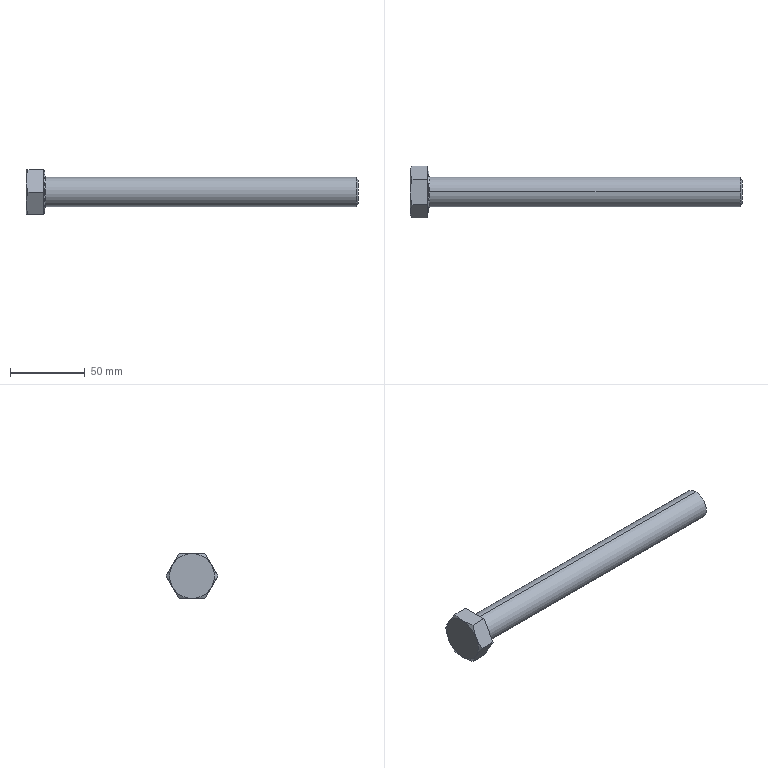Part | SolidWorks | features RevCut 3, Extrusion 1, Fillet 1, LPattern 1, Revolution 1 | 1 solid | 24 faces | box 222.5 x 34.641 x 30 mm | volume 75509 mm3 | cone 10 | plane 10 | torus 2 | cylinder 2 | commonest cylinder face diameters 20 x2
STEP:
#1=CARTESIAN_POINT('',(222.5,0.,7.835));
#2=VERTEX_POINT('',#1);
#3=CARTESIAN_POINT('',(222.5,0.,-7.835));
#4=VERTEX_POINT('',#3);
#5=CARTESIAN_POINT('',(222.5,0.,0.));
#6=DIRECTION('',(-1.,0.,0.));
#7=DIRECTION('',(0.,0.,1.));
#8=AXIS2_PLACEMENT_3D('',#5,#6,#7);
#9=CIRCLE('',#8,7.835);
#10=EDGE_CURVE('',#2,#4,#9,.T.);
#11=ORIENTED_EDGE('',*,*,#10,.T.);
#12=CARTESIAN_POINT('',(221.25,0.,-10.));
#13=VERTEX_POINT('',#12);
#14=CARTESIAN_POINT('',(221.25,0.,-10.));
#15=DIRECTION('',(-0.5,0.,-0.866));
#16=VECTOR('',#15,1000.);
#17=LINE('',#14,#16);
#18=EDGE_CURVE('',#4,#13,#17,.T.);
#19=ORIENTED_EDGE('',*,*,#18,.T.);
#20=CARTESIAN_POINT('',(221.25,0.,10.));
#21=VERTEX_POINT('',#20);
#22=CARTESIAN_POINT('',(221.25,0.,0.));
#23=DIRECTION('',(-1.,0.,0.));
#24=DIRECTION('',(0.,0.,1.));
#25=AXIS2_PLACEMENT_3D('',#22,#23,#24);
#26=CIRCLE('',#25,10.);
#27=EDGE_CURVE('',#21,#13,#26,.T.);
#28=ORIENTED_EDGE('',*,*,#27,.F.);
#29=CARTESIAN_POINT('',(221.25,0.,10.));
#30=DIRECTION('',(-0.5,0.,0.866));
#31=VECTOR('',#30,1000.);
#32=LINE('',#29,#31);
#33=EDGE_CURVE('',#2,#21,#32,.T.);
#34=ORIENTED_EDGE('',*,*,#33,.F.);
#35=EDGE_LOOP('',(#11,#19,#28,#34));
#36=FACE_OUTER_BOUND('',#35,.T.);
#37=CARTESIAN_POINT('',(221.25,0.,0.));
#38=DIRECTION('',(-1.,0.,0.));
#39=DIRECTION('',(0.,0.,1.));
#40=AXIS2_PLACEMENT_3D('',#37,#38,#39);
#41=CONICAL_SURFACE('',#40,10.,1.047);
#42=ADVANCED_FACE('',(#36),#41,.T.);
#43=CARTESIAN_POINT('',(13.3,0.,10.));
#44=VERTEX_POINT('',#43);
#45=CARTESIAN_POINT('',(13.3,0.,-10.));
#46=VERTEX_POINT('',#45);
#47=CARTESIAN_POINT('',(13.3,0.,0.));
#48=DIRECTION('',(1.,0.,0.));
#49=DIRECTION('',(0.,0.,-1.));
#50=AXIS2_PLACEMENT_3D('',#47,#48,#49);
#51=CIRCLE('',#50,10.);
#52=EDGE_CURVE('',#44,#46,#51,.T.);
#53=ORIENTED_EDGE('',*,*,#52,.F.);
#54=CARTESIAN_POINT('',(12.5,0.,10.8));
#55=VERTEX_POINT('',#54);
#56=CARTESIAN_POINT('',(13.3,0.,10.8));
#57=DIRECTION('',(0.,1.,0.));
#58=DIRECTION('',(0.,0.,1.));
#59=AXIS2_PLACEMENT_3D('',#56,#57,#58);
#60=CIRCLE('',#59,0.8);
#61=EDGE_CURVE('',#44,#55,#60,.T.);
#62=ORIENTED_EDGE('',*,*,#61,.T.);
#63=CARTESIAN_POINT('',(12.5,0.,-10.8));
#64=VERTEX_POINT('',#63);
#65=CARTESIAN_POINT('',(12.5,0.,0.));
#66=DIRECTION('',(-1.,0.,0.));
#67=DIRECTION('',(0.,0.,-1.));
#68=AXIS2_PLACEMENT_3D('',#65,#66,#67);
#69=CIRCLE('',#68,10.8);
#70=EDGE_CURVE('',#64,#55,#69,.T.);
#71=ORIENTED_EDGE('',*,*,#70,.F.);
#72=CARTESIAN_POINT('',(13.3,0.,-10.8));
#73=DIRECTION('',(0.,-1.,0.));
#74=DIRECTION('',(0.,0.,-1.));
#75=AXIS2_PLACEMENT_3D('',#72,#73,#74);
#76=CIRCLE('',#75,0.8);
#77=EDGE_CURVE('',#46,#64,#76,.T.);
#78=ORIENTED_EDGE('',*,*,#77,.F.);
#79=EDGE_LOOP('',(#53,#62,#71,#78));
#80=FACE_OUTER_BOUND('',#79,.T.);
#81=CARTESIAN_POINT('',(13.3,0.,0.));
#82=DIRECTION('',(1.,0.,0.));
#83=DIRECTION('',(0.,0.,-1.));
#84=AXIS2_PLACEMENT_3D('',#81,#82,#83);
#85=TOROIDAL_SURFACE('',#84,10.8,0.8);
#86=ADVANCED_FACE('',(#80),#85,.F.);
#87=CARTESIAN_POINT('',(12.5,0.,14.095));
#88=VERTEX_POINT('',#87);
#89=CARTESIAN_POINT('',(12.5,0.,-14.095));
#90=VERTEX_POINT('',#89);
#91=CARTESIAN_POINT('',(12.5,0.,0.));
#92=DIRECTION('',(-1.,0.,0.));
#93=DIRECTION('',(0.,0.,1.));
#94=AXIS2_PLACEMENT_3D('',#91,#92,#93);
#95=CIRCLE('',#94,14.095);
#96=EDGE_CURVE('',#88,#90,#95,.T.);
#97=ORIENTED_EDGE('',*,*,#96,.T.);
#98=CARTESIAN_POINT('',(11.7,0.,-14.557));
#99=VERTEX_POINT('',#98);
#100=CARTESIAN_POINT('',(11.7,0.,-14.557));
#101=DIRECTION('',(-0.866,0.,-0.5));
#102=VECTOR('',#101,1000.);
#103=LINE('',#100,#102);
#104=EDGE_CURVE('',#90,#99,#103,.T.);
#105=ORIENTED_EDGE('',*,*,#104,.T.);
#106=CARTESIAN_POINT('',(11.7,0.,14.557));
#107=VERTEX_POINT('',#106);
#108=CARTESIAN_POINT('',(11.7,0.,0.));
#109=DIRECTION('',(-1.,0.,0.));
#110=DIRECTION('',(0.,0.,1.));
#111=AXIS2_PLACEMENT_3D('',#108,#109,#110);
#112=CIRCLE('',#111,14.557);
#113=EDGE_CURVE('',#107,#99,#112,.T.);
#114=ORIENTED_EDGE('',*,*,#113,.F.);
#115=CARTESIAN_POINT('',(11.7,0.,14.557));
#116=DIRECTION('',(-0.866,0.,0.5));
#117=VECTOR('',#116,1000.);
#118=LINE('',#115,#117);
#119=EDGE_CURVE('',#88,#107,#118,.T.);
#120=ORIENTED_EDGE('',*,*,#119,.F.);
#121=EDGE_LOOP('',(#97,#105,#114,#120));
#122=FACE_OUTER_BOUND('',#121,.T.);
#123=CARTESIAN_POINT('',(11.7,0.,0.));
#124=DIRECTION('',(-1.,0.,0.));
#125=DIRECTION('',(0.,0.,1.));
#126=AXIS2_PLACEMENT_3D('',#123,#124,#125);
#127=CONICAL_SURFACE('',#126,14.557,0.5236);
#128=ADVANCED_FACE('',(#122),#127,.T.);
#129=ORIENTED_EDGE('',*,*,#27,.T.);
#130=CARTESIAN_POINT('',(0.,0.,-10.));
#131=DIRECTION('',(-1.,0.,0.));
#132=VECTOR('',#131,1000.);
#133=LINE('',#130,#132);
#134=EDGE_CURVE('',#13,#46,#133,.T.);
#135=ORIENTED_EDGE('',*,*,#134,.T.);
#136=CARTESIAN_POINT('',(13.3,0.,0.));
#137=DIRECTION('',(1.,0.,0.));
#138=DIRECTION('',(0.,0.,-1.));
#139=AXIS2_PLACEMENT_3D('',#136,#137,#138);
#140=CIRCLE('',#139,10.);
#141=EDGE_CURVE('',#46,#44,#140,.T.);
#142=ORIENTED_EDGE('',*,*,#141,.T.);
#143=CARTESIAN_POINT('',(0.,0.,10.));
#144=DIRECTION('',(-1.,0.,0.));
#145=VECTOR('',#144,1000.);
#146=LINE('',#143,#145);
#147=EDGE_CURVE('',#21,#44,#146,.T.);
#148=ORIENTED_EDGE('',*,*,#147,.F.);
#149=EDGE_LOOP('',(#129,#135,#142,#148));
#150=FACE_OUTER_BOUND('',#149,.T.);
#151=CARTESIAN_POINT('',(0.,0.,0.));
#152=DIRECTION('',(-1.,0.,0.));
#153=DIRECTION('',(0.,0.,1.));
#154=AXIS2_PLACEMENT_3D('',#151,#152,#153);
#155=CYLINDRICAL_SURFACE('',#154,10.);
#156=ADVANCED_FACE('',(#150),#155,.T.);
#157=ORIENTED_EDGE('',*,*,#134,.F.);
#158=CARTESIAN_POINT('',(221.25,0.,0.));
#159=DIRECTION('',(-1.,0.,0.));
#160=DIRECTION('',(0.,0.,1.));
#161=AXIS2_PLACEMENT_3D('',#158,#159,#160);
#162=CIRCLE('',#161,10.);
#163=EDGE_CURVE('',#13,#21,#162,.T.);
#164=ORIENTED_EDGE('',*,*,#163,.T.);
#165=ORIENTED_EDGE('',*,*,#147,.T.);
#166=ORIENTED_EDGE('',*,*,#52,.T.);
#167=EDGE_LOOP('',(#157,#164,#165,#166));
#168=FACE_OUTER_BOUND('',#167,.T.);
#169=CARTESIAN_POINT('',(0.,0.,0.));
#170=DIRECTION('',(-1.,0.,0.));
#171=DIRECTION('',(0.,0.,1.));
#172=AXIS2_PLACEMENT_3D('',#169,#170,#171);
#173=CYLINDRICAL_SURFACE('',#172,10.);
#174=ADVANCED_FACE('',(#168),#173,.T.);
#175=CARTESIAN_POINT('',(11.7,8.66,-15.));
#176=VERTEX_POINT('',#175);
#177=CARTESIAN_POINT('',(11.7,17.321,0.));
#178=VERTEX_POINT('',#177);
#179=CARTESIAN_POINT('',(11.7,8.66,-15.));
#180=DIRECTION('',(0.,0.5,0.866));
#181=VECTOR('',#180,1000.);
#182=LINE('',#179,#181);
#183=EDGE_CURVE('',#176,#178,#182,.T.);
#184=ORIENTED_EDGE('',*,*,#183,.F.);
#185=CARTESIAN_POINT('',(1.34,8.66,-15.));
#186=VERTEX_POINT('',#185);
#187=CARTESIAN_POINT('',(12.5,8.66,-15.));
#188=DIRECTION('',(-1.,0.,0.));
#189=VECTOR('',#188,1000.);
#190=LINE('',#187,#189);
#191=EDGE_CURVE('',#176,#186,#190,.T.);
#192=ORIENTED_EDGE('',*,*,#191,.T.);
#193=CARTESIAN_POINT('',(0.,12.99,-7.5));
#194=VERTEX_POINT('',#193);
#195=CARTESIAN_POINT('',(0.,12.99,-7.5));
#196=CARTESIAN_POINT('',(0.,12.623,-8.136));
#197=CARTESIAN_POINT('',(0.03167,12.254,-8.776));
#198=CARTESIAN_POINT('',(0.1542,11.524,-10.041));
#199=CARTESIAN_POINT('',(0.245,11.161,-10.669));
#200=CARTESIAN_POINT('',(0.595,10.079,-12.542));
#201=CARTESIAN_POINT('',(0.9318,9.367,-13.776));
#202=CARTESIAN_POINT('',(1.34,8.66,-15.));
#203=B_SPLINE_CURVE_WITH_KNOTS('',3,(#195,#196,#197,#198,#199,#200,#201,#202),.UNSPECIFIED.,.F.,.F.,(4,2,2,4),(0.008763,0.01095,0.01313,0.01749),.UNSPECIFIED.);
#204=EDGE_CURVE('',#194,#186,#203,.T.);
#205=ORIENTED_EDGE('',*,*,#204,.F.);
#206=CARTESIAN_POINT('',(1.34,17.321,0.));
#207=VERTEX_POINT('',#206);
#208=CARTESIAN_POINT('',(1.34,17.321,0.));
#209=CARTESIAN_POINT('',(0.9308,16.612,-1.227));
#210=CARTESIAN_POINT('',(0.5939,15.899,-2.463));
#211=CARTESIAN_POINT('',(0.1277,14.457,-4.96));
#212=CARTESIAN_POINT('',(0.,13.728,-6.222));
#213=CARTESIAN_POINT('',(0.,12.99,-7.5));
#214=B_SPLINE_CURVE_WITH_KNOTS('',3,(#208,#209,#210,#211,#212,#213),.UNSPECIFIED.,.F.,.F.,(4,2,4),(0.000000238,0.004382,0.008763),.UNSPECIFIED.);
#215=EDGE_CURVE('',#207,#194,#214,.T.);
#216=ORIENTED_EDGE('',*,*,#215,.F.);
#217=CARTESIAN_POINT('',(12.5,17.321,0.));
#218=DIRECTION('',(-1.,0.,0.));
#219=VECTOR('',#218,1000.);
#220=LINE('',#217,#219);
#221=EDGE_CURVE('',#178,#207,#220,.T.);
#222=ORIENTED_EDGE('',*,*,#221,.F.);
#223=EDGE_LOOP('',(#184,#192,#205,#216,#222));
#224=FACE_OUTER_BOUND('',#223,.T.);
#225=CARTESIAN_POINT('',(12.5,8.66,-15.));
#226=DIRECTION('',(0.,-0.866,0.5));
#227=DIRECTION('',(0.,-0.5,-0.866));
#228=AXIS2_PLACEMENT_3D('',#225,#226,#227);
#229=PLANE('',#228);
#230=ADVANCED_FACE('',(#224),#229,.F.);
#231=CARTESIAN_POINT('',(11.7,8.66,15.));
#232=VERTEX_POINT('',#231);
#233=CARTESIAN_POINT('',(11.7,17.321,0.));
#234=DIRECTION('',(0.,-0.5,0.866));
#235=VECTOR('',#234,1000.);
#236=LINE('',#233,#235);
#237=EDGE_CURVE('',#178,#232,#236,.T.);
#238=ORIENTED_EDGE('',*,*,#237,.F.);
#239=ORIENTED_EDGE('',*,*,#221,.T.);
#240=CARTESIAN_POINT('',(0.,12.99,7.5));
#241=VERTEX_POINT('',#240);
#242=CARTESIAN_POINT('',(0.,12.99,7.5));
#243=CARTESIAN_POINT('',(0.,13.358,6.864));
#244=CARTESIAN_POINT('',(0.03167,13.727,6.224));
#245=CARTESIAN_POINT('',(0.1542,14.457,4.959));
#246=CARTESIAN_POINT('',(0.245,14.82,4.331));
#247=CARTESIAN_POINT('',(0.595,15.901,2.458));
#248=CARTESIAN_POINT('',(0.9318,16.614,1.224));
#249=CARTESIAN_POINT('',(1.34,17.321,0.));
#250=B_SPLINE_CURVE_WITH_KNOTS('',3,(#242,#243,#244,#245,#246,#247,#248,#249),.UNSPECIFIED.,.F.,.F.,(4,2,2,4),(0.008763,0.01095,0.01313,0.01749),.UNSPECIFIED.);
#251=EDGE_CURVE('',#241,#207,#250,.T.);
#252=ORIENTED_EDGE('',*,*,#251,.F.);
#253=CARTESIAN_POINT('',(1.34,8.66,15.));
#254=VERTEX_POINT('',#253);
#255=CARTESIAN_POINT('',(1.34,8.66,15.));
#256=CARTESIAN_POINT('',(0.9308,9.369,13.773));
#257=CARTESIAN_POINT('',(0.5939,10.082,12.537));
#258=CARTESIAN_POINT('',(0.1277,11.524,10.04));
#259=CARTESIAN_POINT('',(0.,12.253,8.778));
#260=CARTESIAN_POINT('',(0.,12.99,7.5));
#261=B_SPLINE_CURVE_WITH_KNOTS('',3,(#255,#256,#257,#258,#259,#260),.UNSPECIFIED.,.F.,.F.,(4,2,4),(0.000000238,0.004382,0.008763),.UNSPECIFIED.);
#262=EDGE_CURVE('',#254,#241,#261,.T.);
#263=ORIENTED_EDGE('',*,*,#262,.F.);
#264=CARTESIAN_POINT('',(12.5,8.66,15.));
#265=DIRECTION('',(-1.,0.,0.));
#266=VECTOR('',#265,1000.);
#267=LINE('',#264,#266);
#268=EDGE_CURVE('',#232,#254,#267,.T.);
#269=ORIENTED_EDGE('',*,*,#268,.F.);
#270=EDGE_LOOP('',(#238,#239,#252,#263,#269));
#271=FACE_OUTER_BOUND('',#270,.T.);
#272=CARTESIAN_POINT('',(12.5,17.321,0.));
#273=DIRECTION('',(0.,-0.866,-0.5));
#274=DIRECTION('',(0.,0.5,-0.866));
#275=AXIS2_PLACEMENT_3D('',#272,#273,#274);
#276=PLANE('',#275);
#277=ADVANCED_FACE('',(#271),#276,.F.);
#278=CARTESIAN_POINT('',(11.7,-8.66,15.));
#279=VERTEX_POINT('',#278);
#280=CARTESIAN_POINT('',(11.7,8.66,15.));
#281=DIRECTION('',(0.,-1.,0.));
#282=VECTOR('',#281,1000.);
#283=LINE('',#280,#282);
#284=EDGE_CURVE('',#232,#279,#283,.T.);
#285=ORIENTED_EDGE('',*,*,#284,.F.);
#286=ORIENTED_EDGE('',*,*,#268,.T.);
#287=CARTESIAN_POINT('',(0.,0.,15.));
#288=VERTEX_POINT('',#287);
#289=CARTESIAN_POINT('',(0.,0.,15.));
#290=CARTESIAN_POINT('',(0.,0.7329,15.));
#291=CARTESIAN_POINT('',(0.03126,1.469,15.));
#292=CARTESIAN_POINT('',(0.1552,2.944,15.));
#293=CARTESIAN_POINT('',(0.2469,3.673,15.));
#294=CARTESIAN_POINT('',(0.5989,5.841,15.));
#295=CARTESIAN_POINT('',(0.9354,7.26,15.));
#296=CARTESIAN_POINT('',(1.34,8.66,15.));
#297=B_SPLINE_CURVE_WITH_KNOTS('',3,(#289,#290,#291,#292,#293,#294,#295,#296),.UNSPECIFIED.,.F.,.F.,(4,2,2,4),(0.02466,0.02686,0.02905,0.03344),.UNSPECIFIED.);
#298=EDGE_CURVE('',#288,#254,#297,.T.);
#299=ORIENTED_EDGE('',*,*,#298,.F.);
#300=CARTESIAN_POINT('',(1.34,-8.66,15.));
#301=VERTEX_POINT('',#300);
#302=CARTESIAN_POINT('',(1.34,-8.66,15.));
#303=CARTESIAN_POINT('',(0.9328,-7.25,15.));
#304=CARTESIAN_POINT('',(0.592,-5.808,15.));
#305=CARTESIAN_POINT('',(0.126,-2.919,15.));
#306=CARTESIAN_POINT('',(0.,-1.465,15.));
#307=CARTESIAN_POINT('',(0.,0.,15.));
#308=B_SPLINE_CURVE_WITH_KNOTS('',3,(#302,#303,#304,#305,#306,#307),.UNSPECIFIED.,.F.,.F.,(4,2,4),(0.0159,0.02028,0.02466),.UNSPECIFIED.);
#309=EDGE_CURVE('',#301,#288,#308,.T.);
#310=ORIENTED_EDGE('',*,*,#309,.F.);
#311=CARTESIAN_POINT('',(12.5,-8.66,15.));
#312=DIRECTION('',(-1.,0.,0.));
#313=VECTOR('',#312,1000.);
#314=LINE('',#311,#313);
#315=EDGE_CURVE('',#279,#301,#314,.T.);
#316=ORIENTED_EDGE('',*,*,#315,.F.);
#317=EDGE_LOOP('',(#285,#286,#299,#310,#316));
#318=FACE_OUTER_BOUND('',#317,.T.);
#319=CARTESIAN_POINT('',(12.5,8.66,15.));
#320=DIRECTION('',(0.,0.,-1.));
#321=DIRECTION('',(-1.,0.,0.));
#322=AXIS2_PLACEMENT_3D('',#319,#320,#321);
#323=PLANE('',#322);
#324=ADVANCED_FACE('',(#318),#323,.F.);
#325=CARTESIAN_POINT('',(11.7,-17.321,0.));
#326=VERTEX_POINT('',#325);
#327=CARTESIAN_POINT('',(11.7,-17.321,0.));
#328=DIRECTION('',(0.,-0.5,-0.866));
#329=VECTOR('',#328,1000.);
#330=LINE('',#327,#329);
#331=EDGE_CURVE('',#279,#326,#330,.T.);
#332=ORIENTED_EDGE('',*,*,#331,.F.);
#333=ORIENTED_EDGE('',*,*,#315,.T.);
#334=CARTESIAN_POINT('',(0.,-12.99,7.5));
#335=VERTEX_POINT('',#334);
#336=CARTESIAN_POINT('',(0.,-12.99,7.5));
#337=CARTESIAN_POINT('',(0.,-12.623,8.136));
#338=CARTESIAN_POINT('',(0.03167,-12.254,8.776));
#339=CARTESIAN_POINT('',(0.1542,-11.524,10.041));
#340=CARTESIAN_POINT('',(0.245,-11.161,10.669));
#341=CARTESIAN_POINT('',(0.595,-10.079,12.542));
#342=CARTESIAN_POINT('',(0.9318,-9.367,13.776));
#343=CARTESIAN_POINT('',(1.34,-8.66,15.));
#344=B_SPLINE_CURVE_WITH_KNOTS('',3,(#336,#337,#338,#339,#340,#341,#342,#343),.UNSPECIFIED.,.F.,.F.,(4,2,2,4),(0.008763,0.01095,0.01313,0.01749),.UNSPECIFIED.);
#345=EDGE_CURVE('',#335,#301,#344,.T.);
#346=ORIENTED_EDGE('',*,*,#345,.F.);
#347=CARTESIAN_POINT('',(1.34,-17.321,0.));
#348=VERTEX_POINT('',#347);
#349=CARTESIAN_POINT('',(1.34,-17.321,0.));
#350=CARTESIAN_POINT('',(0.9308,-16.612,1.227));
#351=CARTESIAN_POINT('',(0.5939,-15.899,2.463));
#352=CARTESIAN_POINT('',(0.1277,-14.457,4.96));
#353=CARTESIAN_POINT('',(0.,-13.728,6.222));
#354=CARTESIAN_POINT('',(0.,-12.99,7.5));
#355=B_SPLINE_CURVE_WITH_KNOTS('',3,(#349,#350,#351,#352,#353,#354),.UNSPECIFIED.,.F.,.F.,(4,2,4),(0.000000238,0.004382,0.008763),.UNSPECIFIED.);
#356=EDGE_CURVE('',#348,#335,#355,.T.);
#357=ORIENTED_EDGE('',*,*,#356,.F.);
#358=CARTESIAN_POINT('',(12.5,-17.321,0.));
#359=DIRECTION('',(-1.,0.,0.));
#360=VECTOR('',#359,1000.);
#361=LINE('',#358,#360);
#362=EDGE_CURVE('',#326,#348,#361,.T.);
#363=ORIENTED_EDGE('',*,*,#362,.F.);
#364=EDGE_LOOP('',(#332,#333,#346,#357,#363));
#365=FACE_OUTER_BOUND('',#364,.T.);
#366=CARTESIAN_POINT('',(12.5,-17.321,0.));
#367=DIRECTION('',(0.,0.866,-0.5));
#368=DIRECTION('',(0.,0.5,0.866));
#369=AXIS2_PLACEMENT_3D('',#366,#367,#368);
#370=PLANE('',#369);
#371=ADVANCED_FACE('',(#365),#370,.F.);
#372=CARTESIAN_POINT('',(11.7,-8.66,-15.));
#373=VERTEX_POINT('',#372);
#374=CARTESIAN_POINT('',(11.7,-8.66,-15.));
#375=DIRECTION('',(0.,0.5,-0.866));
#376=VECTOR('',#375,1000.);
#377=LINE('',#374,#376);
#378=EDGE_CURVE('',#326,#373,#377,.T.);
#379=ORIENTED_EDGE('',*,*,#378,.F.);
#380=ORIENTED_EDGE('',*,*,#362,.T.);
#381=CARTESIAN_POINT('',(0.,-12.99,-7.5));
#382=VERTEX_POINT('',#381);
#383=CARTESIAN_POINT('',(0.,-12.99,-7.5));
#384=CARTESIAN_POINT('',(0.,-13.358,-6.864));
#385=CARTESIAN_POINT('',(0.03167,-13.727,-6.224));
#386=CARTESIAN_POINT('',(0.1542,-14.457,-4.959));
#387=CARTESIAN_POINT('',(0.245,-14.82,-4.331));
#388=CARTESIAN_POINT('',(0.595,-15.901,-2.458));
#389=CARTESIAN_POINT('',(0.9318,-16.614,-1.224));
#390=CARTESIAN_POINT('',(1.34,-17.321,0.));
#391=B_SPLINE_CURVE_WITH_KNOTS('',3,(#383,#384,#385,#386,#387,#388,#389,#390),.UNSPECIFIED.,.F.,.F.,(4,2,2,4),(0.008763,0.01095,0.01313,0.01749),.UNSPECIFIED.);
#392=EDGE_CURVE('',#382,#348,#391,.T.);
#393=ORIENTED_EDGE('',*,*,#392,.F.);
#394=CARTESIAN_POINT('',(1.34,-8.66,-15.));
#395=VERTEX_POINT('',#394);
#396=CARTESIAN_POINT('',(1.34,-8.66,-15.));
#397=CARTESIAN_POINT('',(0.9308,-9.369,-13.773));
#398=CARTESIAN_POINT('',(0.5939,-10.082,-12.537));
#399=CARTESIAN_POINT('',(0.1277,-11.524,-10.04));
#400=CARTESIAN_POINT('',(0.,-12.253,-8.778));
#401=CARTESIAN_POINT('',(0.,-12.99,-7.5));
#402=B_SPLINE_CURVE_WITH_KNOTS('',3,(#396,#397,#398,#399,#400,#401),.UNSPECIFIED.,.F.,.F.,(4,2,4),(0.000000238,0.004382,0.008763),.UNSPECIFIED.);
#403=EDGE_CURVE('',#395,#382,#402,.T.);
#404=ORIENTED_EDGE('',*,*,#403,.F.);
#405=CARTESIAN_POINT('',(12.5,-8.66,-15.));
#406=DIRECTION('',(-1.,0.,0.));
#407=VECTOR('',#406,1000.);
#408=LINE('',#405,#407);
#409=EDGE_CURVE('',#373,#395,#408,.T.);
#410=ORIENTED_EDGE('',*,*,#409,.F.);
#411=EDGE_LOOP('',(#379,#380,#393,#404,#410));
#412=FACE_OUTER_BOUND('',#411,.T.);
#413=CARTESIAN_POINT('',(12.5,-8.66,-15.));
#414=DIRECTION('',(0.,0.866,0.5));
#415=DIRECTION('',(0.,-0.5,0.866));
#416=AXIS2_PLACEMENT_3D('',#413,#414,#415);
#417=PLANE('',#416);
#418=ADVANCED_FACE('',(#412),#417,.F.);
#419=CARTESIAN_POINT('',(11.7,8.66,-15.));
#420=DIRECTION('',(0.,1.,0.));
#421=VECTOR('',#420,1000.);
#422=LINE('',#419,#421);
#423=EDGE_CURVE('',#373,#176,#422,.T.);
#424=ORIENTED_EDGE('',*,*,#423,.F.);
#425=ORIENTED_EDGE('',*,*,#409,.T.);
#426=CARTESIAN_POINT('',(0.,0.,-15.));
#427=VERTEX_POINT('',#426);
#428=CARTESIAN_POINT('',(0.,0.,-15.));
#429=CARTESIAN_POINT('',(0.,-1.465,-15.));
#430=CARTESIAN_POINT('',(0.126,-2.919,-15.));
#431=CARTESIAN_POINT('',(0.592,-5.808,-15.));
#432=CARTESIAN_POINT('',(0.9328,-7.25,-15.));
#433=CARTESIAN_POINT('',(1.34,-8.66,-15.));
#434=B_SPLINE_CURVE_WITH_KNOTS('',3,(#428,#429,#430,#431,#432,#433),.UNSPECIFIED.,.F.,.F.,(4,2,4),(0.04846,0.05285,0.05723),.UNSPECIFIED.);
#435=EDGE_CURVE('',#427,#395,#434,.T.);
#436=ORIENTED_EDGE('',*,*,#435,.F.);
#437=CARTESIAN_POINT('',(1.34,8.66,-15.));
#438=CARTESIAN_POINT('',(0.9354,7.26,-15.));
#439=CARTESIAN_POINT('',(0.5989,5.841,-15.));
#440=CARTESIAN_POINT('',(0.2469,3.673,-15.));
#441=CARTESIAN_POINT('',(0.1552,2.944,-15.));
#442=CARTESIAN_POINT('',(0.03126,1.469,-15.));
#443=CARTESIAN_POINT('',(0.,0.7329,-15.));
#444=CARTESIAN_POINT('',(0.,0.,-15.));
#445=B_SPLINE_CURVE_WITH_KNOTS('',3,(#437,#438,#439,#440,#441,#442,#443,#444),.UNSPECIFIED.,.F.,.F.,(4,2,2,4),(0.03969,0.04407,0.04627,0.04846),.UNSPECIFIED.);
#446=EDGE_CURVE('',#186,#427,#445,.T.);
#447=ORIENTED_EDGE('',*,*,#446,.F.);
#448=ORIENTED_EDGE('',*,*,#191,.F.);
#449=EDGE_LOOP('',(#424,#425,#436,#447,#448));
#450=FACE_OUTER_BOUND('',#449,.T.);
#451=CARTESIAN_POINT('',(12.5,8.66,-15.));
#452=DIRECTION('',(0.,0.,1.));
#453=DIRECTION('',(0.,-1.,0.));
#454=AXIS2_PLACEMENT_3D('',#451,#452,#453);
#455=PLANE('',#454);
#456=ADVANCED_FACE('',(#450),#455,.F.);
#457=ORIENTED_EDGE('',*,*,#403,.T.);
#458=CARTESIAN_POINT('',(0.,0.,0.));
#459=DIRECTION('',(1.,0.,0.));
#460=DIRECTION('',(0.,0.,-1.));
#461=AXIS2_PLACEMENT_3D('',#458,#459,#460);
#462=CIRCLE('',#461,15.);
#463=EDGE_CURVE('',#382,#427,#462,.T.);
#464=ORIENTED_EDGE('',*,*,#463,.T.);
#465=ORIENTED_EDGE('',*,*,#435,.T.);
#466=EDGE_LOOP('',(#457,#464,#465));
#467=FACE_OUTER_BOUND('',#466,.T.);
#468=CARTESIAN_POINT('',(0.,0.,0.));
#469=DIRECTION('',(1.,0.,0.));
#470=DIRECTION('',(0.,0.,-1.));
#471=AXIS2_PLACEMENT_3D('',#468,#469,#470);
#472=CONICAL_SURFACE('',#471,15.,1.047);
#473=ADVANCED_FACE('',(#467),#472,.T.);
#474=ORIENTED_EDGE('',*,*,#356,.T.);
#475=CARTESIAN_POINT('',(0.,0.,0.));
#476=DIRECTION('',(1.,0.,0.));
#477=DIRECTION('',(0.,0.,-1.));
#478=AXIS2_PLACEMENT_3D('',#475,#476,#477);
#479=CIRCLE('',#478,15.);
#480=EDGE_CURVE('',#335,#382,#479,.T.);
#481=ORIENTED_EDGE('',*,*,#480,.T.);
#482=ORIENTED_EDGE('',*,*,#392,.T.);
#483=EDGE_LOOP('',(#474,#481,#482));
#484=FACE_OUTER_BOUND('',#483,.T.);
#485=CARTESIAN_POINT('',(0.,0.,0.));
#486=DIRECTION('',(1.,0.,0.));
#487=DIRECTION('',(0.,0.,-1.));
#488=AXIS2_PLACEMENT_3D('',#485,#486,#487);
#489=CONICAL_SURFACE('',#488,15.,1.047);
#490=ADVANCED_FACE('',(#484),#489,.T.);
#491=ORIENTED_EDGE('',*,*,#309,.T.);
#492=CARTESIAN_POINT('',(0.,0.,0.));
#493=DIRECTION('',(1.,0.,0.));
#494=DIRECTION('',(0.,0.,-1.));
#495=AXIS2_PLACEMENT_3D('',#492,#493,#494);
#496=CIRCLE('',#495,15.);
#497=EDGE_CURVE('',#288,#335,#496,.T.);
#498=ORIENTED_EDGE('',*,*,#497,.T.);
#499=ORIENTED_EDGE('',*,*,#345,.T.);
#500=EDGE_LOOP('',(#491,#498,#499));
#501=FACE_OUTER_BOUND('',#500,.T.);
#502=CARTESIAN_POINT('',(0.,0.,0.));
#503=DIRECTION('',(1.,0.,0.));
#504=DIRECTION('',(0.,0.,-1.));
#505=AXIS2_PLACEMENT_3D('',#502,#503,#504);
#506=CONICAL_SURFACE('',#505,15.,1.047);
#507=ADVANCED_FACE('',(#501),#506,.T.);
#508=ORIENTED_EDGE('',*,*,#298,.T.);
#509=ORIENTED_EDGE('',*,*,#262,.T.);
#510=CARTESIAN_POINT('',(0.,0.,0.));
#511=DIRECTION('',(-1.,0.,0.));
#512=DIRECTION('',(0.,0.,1.));
#513=AXIS2_PLACEMENT_3D('',#510,#511,#512);
#514=CIRCLE('',#513,15.);
#515=EDGE_CURVE('',#288,#241,#514,.T.);
#516=ORIENTED_EDGE('',*,*,#515,.F.);
#517=EDGE_LOOP('',(#508,#509,#516));
#518=FACE_OUTER_BOUND('',#517,.T.);
#519=CARTESIAN_POINT('',(0.,0.,0.));
#520=DIRECTION('',(1.,0.,0.));
#521=DIRECTION('',(0.,0.,-1.));
#522=AXIS2_PLACEMENT_3D('',#519,#520,#521);
#523=CONICAL_SURFACE('',#522,15.,1.047);
#524=ADVANCED_FACE('',(#518),#523,.T.);
#525=ORIENTED_EDGE('',*,*,#251,.T.);
#526=ORIENTED_EDGE('',*,*,#215,.T.);
#527=CARTESIAN_POINT('',(0.,0.,0.));
#528=DIRECTION('',(1.,0.,0.));
#529=DIRECTION('',(0.,0.,-1.));
#530=AXIS2_PLACEMENT_3D('',#527,#528,#529);
#531=CIRCLE('',#530,15.);
#532=EDGE_CURVE('',#194,#241,#531,.T.);
#533=ORIENTED_EDGE('',*,*,#532,.T.);
#534=EDGE_LOOP('',(#525,#526,#533));
#535=FACE_OUTER_BOUND('',#534,.T.);
#536=CARTESIAN_POINT('',(0.,0.,0.));
#537=DIRECTION('',(1.,0.,0.));
#538=DIRECTION('',(0.,0.,-1.));
#539=AXIS2_PLACEMENT_3D('',#536,#537,#538);
#540=CONICAL_SURFACE('',#539,15.,1.047);
#541=ADVANCED_FACE('',(#535),#540,.T.);
#542=ORIENTED_EDGE('',*,*,#204,.T.);
#543=ORIENTED_EDGE('',*,*,#446,.T.);
#544=CARTESIAN_POINT('',(0.,0.,0.));
#545=DIRECTION('',(1.,0.,0.));
#546=DIRECTION('',(0.,0.,-1.));
#547=AXIS2_PLACEMENT_3D('',#544,#545,#546);
#548=CIRCLE('',#547,15.);
#549=EDGE_CURVE('',#427,#194,#548,.T.);
#550=ORIENTED_EDGE('',*,*,#549,.T.);
#551=EDGE_LOOP('',(#542,#543,#550));
#552=FACE_OUTER_BOUND('',#551,.T.);
#553=CARTESIAN_POINT('',(0.,0.,0.));
#554=DIRECTION('',(1.,0.,0.));
#555=DIRECTION('',(0.,0.,-1.));
#556=AXIS2_PLACEMENT_3D('',#553,#554,#555);
#557=CONICAL_SURFACE('',#556,15.,1.047);
#558=ADVANCED_FACE('',(#552),#557,.T.);
#559=ORIENTED_EDGE('',*,*,#549,.F.);
#560=ORIENTED_EDGE('',*,*,#463,.F.);
#561=ORIENTED_EDGE('',*,*,#480,.F.);
#562=ORIENTED_EDGE('',*,*,#497,.F.);
#563=ORIENTED_EDGE('',*,*,#515,.T.);
#564=ORIENTED_EDGE('',*,*,#532,.F.);
#565=EDGE_LOOP('',(#559,#560,#561,#562,#563,#564));
#566=FACE_OUTER_BOUND('',#565,.T.);
#567=CARTESIAN_POINT('',(0.,17.321,0.));
#568=DIRECTION('',(1.,0.,0.));
#569=DIRECTION('',(0.,0.,-1.));
#570=AXIS2_PLACEMENT_3D('',#567,#568,#569);
#571=PLANE('',#570);
#572=ADVANCED_FACE('',(#566),#571,.F.);
#573=ORIENTED_EDGE('',*,*,#113,.T.);
#574=CARTESIAN_POINT('',(11.7,0.,0.));
#575=DIRECTION('',(-1.,0.,0.));
#576=DIRECTION('',(0.,0.,1.));
#577=AXIS2_PLACEMENT_3D('',#574,#575,#576);
#578=CIRCLE('',#577,14.557);
#579=EDGE_CURVE('',#99,#107,#578,.T.);
#580=ORIENTED_EDGE('',*,*,#579,.T.);
#581=EDGE_LOOP('',(#573,#580));
#582=FACE_BOUND('',#581,.T.);
#583=ORIENTED_EDGE('',*,*,#183,.T.);
#584=ORIENTED_EDGE('',*,*,#237,.T.);
#585=ORIENTED_EDGE('',*,*,#284,.T.);
#586=ORIENTED_EDGE('',*,*,#331,.T.);
#587=ORIENTED_EDGE('',*,*,#378,.T.);
#588=ORIENTED_EDGE('',*,*,#423,.T.);
#589=EDGE_LOOP('',(#583,#584,#585,#586,#587,#588));
#590=FACE_OUTER_BOUND('',#589,.T.);
#591=CARTESIAN_POINT('',(11.7,14.557,0.));
#592=DIRECTION('',(1.,0.,0.));
#593=DIRECTION('',(0.,0.,-1.));
#594=AXIS2_PLACEMENT_3D('',#591,#592,#593);
#595=PLANE('',#594);
#596=ADVANCED_FACE('',(#582,#590),#595,.T.);
#597=ORIENTED_EDGE('',*,*,#104,.F.);
#598=CARTESIAN_POINT('',(12.5,0.,0.));
#599=DIRECTION('',(-1.,0.,0.));
#600=DIRECTION('',(0.,0.,1.));
#601=AXIS2_PLACEMENT_3D('',#598,#599,#600);
#602=CIRCLE('',#601,14.095);
#603=EDGE_CURVE('',#90,#88,#602,.T.);
#604=ORIENTED_EDGE('',*,*,#603,.T.);
#605=ORIENTED_EDGE('',*,*,#119,.T.);
#606=ORIENTED_EDGE('',*,*,#579,.F.);
#607=EDGE_LOOP('',(#597,#604,#605,#606));
#608=FACE_OUTER_BOUND('',#607,.T.);
#609=CARTESIAN_POINT('',(11.7,0.,0.));
#610=DIRECTION('',(-1.,0.,0.));
#611=DIRECTION('',(0.,0.,1.));
#612=AXIS2_PLACEMENT_3D('',#609,#610,#611);
#613=CONICAL_SURFACE('',#612,14.557,0.5236);
#614=ADVANCED_FACE('',(#608),#613,.T.);
#615=ORIENTED_EDGE('',*,*,#70,.T.);
#616=CARTESIAN_POINT('',(12.5,0.,0.));
#617=DIRECTION('',(-1.,0.,0.));
#618=DIRECTION('',(0.,0.,-1.));
#619=AXIS2_PLACEMENT_3D('',#616,#617,#618);
#620=CIRCLE('',#619,10.8);
#621=EDGE_CURVE('',#55,#64,#620,.T.);
#622=ORIENTED_EDGE('',*,*,#621,.T.);
#623=EDGE_LOOP('',(#615,#622));
#624=FACE_BOUND('',#623,.T.);
#625=ORIENTED_EDGE('',*,*,#96,.F.);
#626=ORIENTED_EDGE('',*,*,#603,.F.);
#627=EDGE_LOOP('',(#625,#626));
#628=FACE_OUTER_BOUND('',#627,.T.);
#629=CARTESIAN_POINT('',(12.5,17.321,0.));
#630=DIRECTION('',(1.,0.,0.));
#631=DIRECTION('',(0.,0.,-1.));
#632=AXIS2_PLACEMENT_3D('',#629,#630,#631);
#633=PLANE('',#632);
#634=ADVANCED_FACE('',(#624,#628),#633,.T.);
#635=ORIENTED_EDGE('',*,*,#61,.F.);
#636=ORIENTED_EDGE('',*,*,#141,.F.);
#637=ORIENTED_EDGE('',*,*,#77,.T.);
#638=ORIENTED_EDGE('',*,*,#621,.F.);
#639=EDGE_LOOP('',(#635,#636,#637,#638));
#640=FACE_OUTER_BOUND('',#639,.T.);
#641=CARTESIAN_POINT('',(13.3,0.,0.));
#642=DIRECTION('',(1.,0.,0.));
#643=DIRECTION('',(0.,0.,-1.));
#644=AXIS2_PLACEMENT_3D('',#641,#642,#643);
#645=TOROIDAL_SURFACE('',#644,10.8,0.8);
#646=ADVANCED_FACE('',(#640),#645,.F.);
#647=ORIENTED_EDGE('',*,*,#18,.F.);
#648=CARTESIAN_POINT('',(222.5,0.,0.));
#649=DIRECTION('',(-1.,0.,0.));
#650=DIRECTION('',(0.,0.,1.));
#651=AXIS2_PLACEMENT_3D('',#648,#649,#650);
#652=CIRCLE('',#651,7.835);
#653=EDGE_CURVE('',#4,#2,#652,.T.);
#654=ORIENTED_EDGE('',*,*,#653,.T.);
#655=ORIENTED_EDGE('',*,*,#33,.T.);
#656=ORIENTED_EDGE('',*,*,#163,.F.);
#657=EDGE_LOOP('',(#647,#654,#655,#656));
#658=FACE_OUTER_BOUND('',#657,.T.);
#659=CARTESIAN_POINT('',(221.25,0.,0.));
#660=DIRECTION('',(-1.,0.,0.));
#661=DIRECTION('',(0.,0.,1.));
#662=AXIS2_PLACEMENT_3D('',#659,#660,#661);
#663=CONICAL_SURFACE('',#662,10.,1.047);
#664=ADVANCED_FACE('',(#658),#663,.T.);
#665=ORIENTED_EDGE('',*,*,#10,.F.);
#666=ORIENTED_EDGE('',*,*,#653,.F.);
#667=EDGE_LOOP('',(#665,#666));
#668=FACE_OUTER_BOUND('',#667,.T.);
#669=CARTESIAN_POINT('',(222.5,0.,0.));
#670=DIRECTION('',(-1.,0.,0.));
#671=DIRECTION('',(0.,0.,1.));
#672=AXIS2_PLACEMENT_3D('',#669,#670,#671);
#673=PLANE('',#672);
#674=ADVANCED_FACE('',(#668),#673,.F.);
#675=CLOSED_SHELL('',(#42,#86,#128,#156,#174,#230,#277,#324,#371,#418,#456,#473,#490,#507,#524,#541,#558,#572,#596,#614,#634,#646,#664,#674));
#676=MANIFOLD_SOLID_BREP('',#675);
#677=CARTESIAN_POINT('',(0.,0.,0.));
#678=DIRECTION('',(0.,0.,1.));
#679=DIRECTION('',(1.,0.,0.));
#680=AXIS2_PLACEMENT_3D('',#677,#678,#679);
#681=(LENGTH_UNIT()NAMED_UNIT(*)SI_UNIT(.MILLI.,.METRE.));
#682=UNCERTAINTY_MEASURE_WITH_UNIT(LENGTH_MEASURE(0.00001),#681,'','');
#683=(NAMED_UNIT(*)PLANE_ANGLE_UNIT()SI_UNIT($,.RADIAN.));
#684=(NAMED_UNIT(*)SI_UNIT($,.STERADIAN.)SOLID_ANGLE_UNIT());
#685=(GEOMETRIC_REPRESENTATION_CONTEXT(3)GLOBAL_UNCERTAINTY_ASSIGNED_CONTEXT((#682))GLOBAL_UNIT_ASSIGNED_CONTEXT((#681,#683,#684))REPRESENTATION_CONTEXT('',''));
#686=ADVANCED_BREP_SHAPE_REPRESENTATION('',(#676,#680),#685);